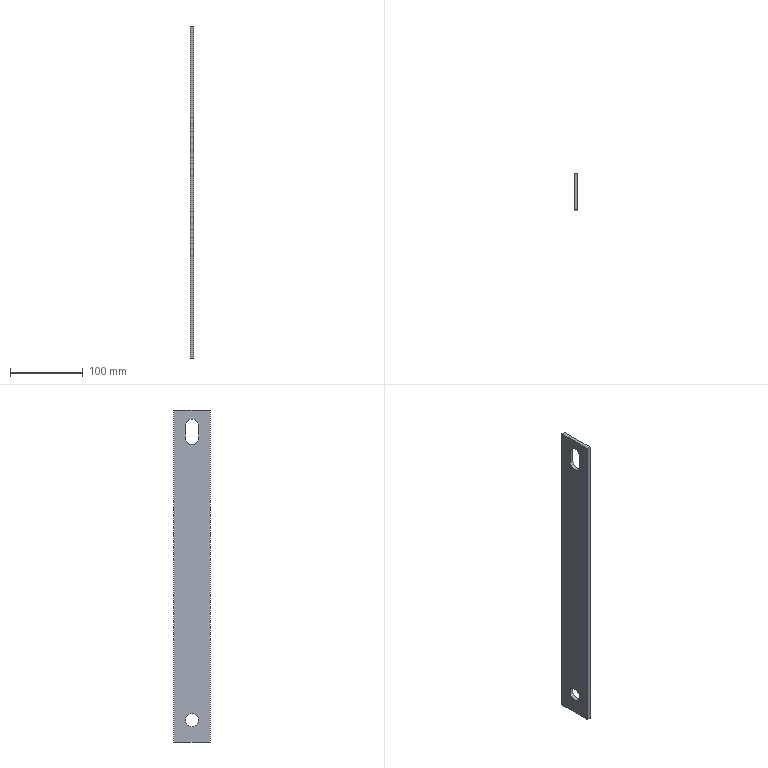Part | NX | features MAIN_BODY 2 | 1 solid | 11 faces | box 5 x 50 x 455 mm | volume 109675 mm3 | plane 8 | cylinder 3 | commonest cylinder face diameters 18 x3
STEP:
#1=CARTESIAN_POINT('',(1560.,-656.,343.5));
#2=VERTEX_POINT('',#1);
#3=CARTESIAN_POINT('',(1560.,-674.,343.5));
#4=VERTEX_POINT('',#3);
#5=CARTESIAN_POINT('',(1560.,-665.,343.5));
#6=DIRECTION('',(-1.,0.,0.));
#7=DIRECTION('',(0.,0.,-1.));
#8=AXIS2_PLACEMENT_3D('',#5,#6,#7);
#9=CIRCLE('',#8,9.);
#10=EDGE_CURVE('',#2,#4,#9,.F.);
#11=ORIENTED_EDGE('',*,*,#10,.F.);
#12=CARTESIAN_POINT('',(1565.,-656.,343.5));
#13=VERTEX_POINT('',#12);
#14=CARTESIAN_POINT('',(1563.,-656.,343.5));
#15=DIRECTION('',(-1.,0.,0.));
#16=VECTOR('',#15,1000.);
#17=LINE('',#14,#16);
#18=EDGE_CURVE('',#13,#2,#17,.T.);
#19=ORIENTED_EDGE('',*,*,#18,.F.);
#20=CARTESIAN_POINT('',(1565.,-674.,343.5));
#21=VERTEX_POINT('',#20);
#22=CARTESIAN_POINT('',(1565.,-665.,343.5));
#23=DIRECTION('',(-1.,0.,0.));
#24=DIRECTION('',(0.,0.,-1.));
#25=AXIS2_PLACEMENT_3D('',#22,#23,#24);
#26=CIRCLE('',#25,9.);
#27=EDGE_CURVE('',#13,#21,#26,.F.);
#28=ORIENTED_EDGE('',*,*,#27,.T.);
#29=CARTESIAN_POINT('',(1563.,-674.,343.5));
#30=DIRECTION('',(-1.,0.,0.));
#31=VECTOR('',#30,1000.);
#32=LINE('',#29,#31);
#33=EDGE_CURVE('',#21,#4,#32,.T.);
#34=ORIENTED_EDGE('',*,*,#33,.T.);
#35=EDGE_LOOP('',(#11,#19,#28,#34));
#36=FACE_BOUND('',#35,.T.);
#37=CARTESIAN_POINT('',(1563.,-665.,343.5));
#38=DIRECTION('',(-1.,0.,0.));
#39=DIRECTION('',(0.,1.,0.));
#40=AXIS2_PLACEMENT_3D('',#37,#38,#39);
#41=CYLINDRICAL_SURFACE('',#40,9.);
#42=ADVANCED_FACE('',(#36),#41,.F.);
#43=CARTESIAN_POINT('',(1560.,-656.,326.5));
#44=VERTEX_POINT('',#43);
#45=CARTESIAN_POINT('',(1560.,-656.,206.25));
#46=DIRECTION('',(0.,0.,-1.));
#47=VECTOR('',#46,1000.);
#48=LINE('',#45,#47);
#49=EDGE_CURVE('',#2,#44,#48,.T.);
#50=ORIENTED_EDGE('',*,*,#49,.T.);
#51=CARTESIAN_POINT('',(1565.,-656.,326.5));
#52=VERTEX_POINT('',#51);
#53=CARTESIAN_POINT('',(1563.,-656.,326.5));
#54=DIRECTION('',(-1.,0.,0.));
#55=VECTOR('',#54,1000.);
#56=LINE('',#53,#55);
#57=EDGE_CURVE('',#52,#44,#56,.T.);
#58=ORIENTED_EDGE('',*,*,#57,.F.);
#59=CARTESIAN_POINT('',(1565.,-656.,206.25));
#60=DIRECTION('',(0.,0.,-1.));
#61=VECTOR('',#60,1000.);
#62=LINE('',#59,#61);
#63=EDGE_CURVE('',#13,#52,#62,.T.);
#64=ORIENTED_EDGE('',*,*,#63,.F.);
#65=ORIENTED_EDGE('',*,*,#18,.T.);
#66=EDGE_LOOP('',(#50,#58,#64,#65));
#67=FACE_BOUND('',#66,.T.);
#68=CARTESIAN_POINT('',(1563.,-656.,206.25));
#69=DIRECTION('',(0.,-1.,0.));
#70=DIRECTION('',(-1.,0.,0.));
#71=AXIS2_PLACEMENT_3D('',#68,#69,#70);
#72=PLANE('',#71);
#73=ADVANCED_FACE('',(#67),#72,.T.);
#74=CARTESIAN_POINT('',(1560.,-674.,326.5));
#75=VERTEX_POINT('',#74);
#76=CARTESIAN_POINT('',(1560.,-665.,326.5));
#77=DIRECTION('',(-1.,0.,0.));
#78=DIRECTION('',(0.,0.,-1.));
#79=AXIS2_PLACEMENT_3D('',#76,#77,#78);
#80=CIRCLE('',#79,9.);
#81=EDGE_CURVE('',#75,#44,#80,.F.);
#82=ORIENTED_EDGE('',*,*,#81,.F.);
#83=CARTESIAN_POINT('',(1565.,-674.,326.5));
#84=VERTEX_POINT('',#83);
#85=CARTESIAN_POINT('',(1563.,-674.,326.5));
#86=DIRECTION('',(1.,0.,0.));
#87=VECTOR('',#86,1000.);
#88=LINE('',#85,#87);
#89=EDGE_CURVE('',#84,#75,#88,.F.);
#90=ORIENTED_EDGE('',*,*,#89,.F.);
#91=CARTESIAN_POINT('',(1565.,-665.,326.5));
#92=DIRECTION('',(-1.,0.,0.));
#93=DIRECTION('',(0.,0.,-1.));
#94=AXIS2_PLACEMENT_3D('',#91,#92,#93);
#95=CIRCLE('',#94,9.);
#96=EDGE_CURVE('',#84,#52,#95,.F.);
#97=ORIENTED_EDGE('',*,*,#96,.T.);
#98=ORIENTED_EDGE('',*,*,#57,.T.);
#99=EDGE_LOOP('',(#82,#90,#97,#98));
#100=FACE_BOUND('',#99,.T.);
#101=CARTESIAN_POINT('',(1563.,-665.,326.5));
#102=DIRECTION('',(-1.,0.,0.));
#103=DIRECTION('',(0.,1.,0.));
#104=AXIS2_PLACEMENT_3D('',#101,#102,#103);
#105=CYLINDRICAL_SURFACE('',#104,9.);
#106=ADVANCED_FACE('',(#100),#105,.F.);
#107=CARTESIAN_POINT('',(1560.,-640.,-90.));
#108=VERTEX_POINT('',#107);
#109=CARTESIAN_POINT('',(1560.,-640.,365.));
#110=VERTEX_POINT('',#109);
#111=CARTESIAN_POINT('',(1560.,-640.,220.));
#112=DIRECTION('',(0.,0.,1.));
#113=VECTOR('',#112,1000.);
#114=LINE('',#111,#113);
#115=EDGE_CURVE('',#108,#110,#114,.T.);
#116=ORIENTED_EDGE('',*,*,#115,.T.);
#117=CARTESIAN_POINT('',(1565.,-640.,365.));
#118=VERTEX_POINT('',#117);
#119=CARTESIAN_POINT('',(1563.,-640.,365.));
#120=DIRECTION('',(-1.,0.,0.));
#121=VECTOR('',#120,1000.);
#122=LINE('',#119,#121);
#123=EDGE_CURVE('',#118,#110,#122,.T.);
#124=ORIENTED_EDGE('',*,*,#123,.F.);
#125=CARTESIAN_POINT('',(1565.,-640.,-90.));
#126=VERTEX_POINT('',#125);
#127=CARTESIAN_POINT('',(1565.,-640.,-80.));
#128=DIRECTION('',(0.,0.,1.));
#129=VECTOR('',#128,1000.);
#130=LINE('',#127,#129);
#131=EDGE_CURVE('',#126,#118,#130,.T.);
#132=ORIENTED_EDGE('',*,*,#131,.F.);
#133=CARTESIAN_POINT('',(1563.,-640.,-90.));
#134=DIRECTION('',(-1.,0.,0.));
#135=VECTOR('',#134,1000.);
#136=LINE('',#133,#135);
#137=EDGE_CURVE('',#126,#108,#136,.T.);
#138=ORIENTED_EDGE('',*,*,#137,.T.);
#139=EDGE_LOOP('',(#116,#124,#132,#138));
#140=FACE_BOUND('',#139,.T.);
#141=CARTESIAN_POINT('',(1563.,-640.,-80.));
#142=DIRECTION('',(0.,1.,0.));
#143=DIRECTION('',(0.,0.,1.));
#144=AXIS2_PLACEMENT_3D('',#141,#142,#143);
#145=PLANE('',#144);
#146=ADVANCED_FACE('',(#140),#145,.T.);
#147=CARTESIAN_POINT('',(1560.,-690.,365.));
#148=VERTEX_POINT('',#147);
#149=CARTESIAN_POINT('',(1560.,-647.5,365.));
#150=DIRECTION('',(0.,-1.,0.));
#151=VECTOR('',#150,1000.);
#152=LINE('',#149,#151);
#153=EDGE_CURVE('',#110,#148,#152,.T.);
#154=ORIENTED_EDGE('',*,*,#153,.T.);
#155=CARTESIAN_POINT('',(1565.,-690.,365.));
#156=VERTEX_POINT('',#155);
#157=CARTESIAN_POINT('',(1563.,-690.,365.));
#158=DIRECTION('',(-1.,0.,0.));
#159=VECTOR('',#158,1000.);
#160=LINE('',#157,#159);
#161=EDGE_CURVE('',#156,#148,#160,.T.);
#162=ORIENTED_EDGE('',*,*,#161,.F.);
#163=CARTESIAN_POINT('',(1565.,-647.5,365.));
#164=DIRECTION('',(0.,-1.,0.));
#165=VECTOR('',#164,1000.);
#166=LINE('',#163,#165);
#167=EDGE_CURVE('',#118,#156,#166,.T.);
#168=ORIENTED_EDGE('',*,*,#167,.F.);
#169=ORIENTED_EDGE('',*,*,#123,.T.);
#170=EDGE_LOOP('',(#154,#162,#168,#169));
#171=FACE_BOUND('',#170,.T.);
#172=CARTESIAN_POINT('',(1563.,-647.5,365.));
#173=DIRECTION('',(0.,0.,1.));
#174=DIRECTION('',(-1.,0.,0.));
#175=AXIS2_PLACEMENT_3D('',#172,#173,#174);
#176=PLANE('',#175);
#177=ADVANCED_FACE('',(#171),#176,.T.);
#178=CARTESIAN_POINT('',(1560.,-690.,-90.));
#179=VERTEX_POINT('',#178);
#180=CARTESIAN_POINT('',(1560.,-690.,220.));
#181=DIRECTION('',(0.,0.,-1.));
#182=VECTOR('',#181,1000.);
#183=LINE('',#180,#182);
#184=EDGE_CURVE('',#148,#179,#183,.T.);
#185=ORIENTED_EDGE('',*,*,#184,.T.);
#186=CARTESIAN_POINT('',(1565.,-690.,-90.));
#187=VERTEX_POINT('',#186);
#188=CARTESIAN_POINT('',(1563.,-690.,-90.));
#189=DIRECTION('',(-1.,0.,0.));
#190=VECTOR('',#189,1000.);
#191=LINE('',#188,#190);
#192=EDGE_CURVE('',#187,#179,#191,.T.);
#193=ORIENTED_EDGE('',*,*,#192,.F.);
#194=CARTESIAN_POINT('',(1565.,-690.,220.));
#195=DIRECTION('',(0.,0.,-1.));
#196=VECTOR('',#195,1000.);
#197=LINE('',#194,#196);
#198=EDGE_CURVE('',#156,#187,#197,.T.);
#199=ORIENTED_EDGE('',*,*,#198,.F.);
#200=ORIENTED_EDGE('',*,*,#161,.T.);
#201=EDGE_LOOP('',(#185,#193,#199,#200));
#202=FACE_BOUND('',#201,.T.);
#203=CARTESIAN_POINT('',(1563.,-690.,220.));
#204=DIRECTION('',(0.,-1.,0.));
#205=DIRECTION('',(0.,0.,-1.));
#206=AXIS2_PLACEMENT_3D('',#203,#204,#205);
#207=PLANE('',#206);
#208=ADVANCED_FACE('',(#202),#207,.T.);
#209=CARTESIAN_POINT('',(1565.,-665.,-69.));
#210=VERTEX_POINT('',#209);
#211=CARTESIAN_POINT('',(1565.,-665.,-60.));
#212=DIRECTION('',(-1.,0.,0.));
#213=DIRECTION('',(0.,0.,-1.));
#214=AXIS2_PLACEMENT_3D('',#211,#212,#213);
#215=CIRCLE('',#214,9.);
#216=EDGE_CURVE('',#210,#210,#215,.F.);
#217=ORIENTED_EDGE('',*,*,#216,.T.);
#218=EDGE_LOOP('',(#217));
#219=FACE_BOUND('',#218,.T.);
#220=CARTESIAN_POINT('',(1560.,-665.,-69.));
#221=VERTEX_POINT('',#220);
#222=CARTESIAN_POINT('',(1560.,-665.,-60.));
#223=DIRECTION('',(-1.,0.,0.));
#224=DIRECTION('',(0.,0.,-1.));
#225=AXIS2_PLACEMENT_3D('',#222,#223,#224);
#226=CIRCLE('',#225,9.);
#227=EDGE_CURVE('',#221,#221,#226,.F.);
#228=ORIENTED_EDGE('',*,*,#227,.F.);
#229=EDGE_LOOP('',(#228));
#230=FACE_BOUND('',#229,.T.);
#231=CARTESIAN_POINT('',(1563.,-665.,-60.));
#232=DIRECTION('',(-1.,0.,0.));
#233=DIRECTION('',(0.,1.,0.));
#234=AXIS2_PLACEMENT_3D('',#231,#232,#233);
#235=CYLINDRICAL_SURFACE('',#234,9.);
#236=ADVANCED_FACE('',(#219,#230),#235,.F.);
#237=CARTESIAN_POINT('',(1560.,-647.5,-90.));
#238=DIRECTION('',(0.,1.,0.));
#239=VECTOR('',#238,1000.);
#240=LINE('',#237,#239);
#241=EDGE_CURVE('',#179,#108,#240,.T.);
#242=ORIENTED_EDGE('',*,*,#241,.T.);
#243=ORIENTED_EDGE('',*,*,#137,.F.);
#244=CARTESIAN_POINT('',(1565.,-682.5,-90.));
#245=DIRECTION('',(0.,1.,0.));
#246=VECTOR('',#245,1000.);
#247=LINE('',#244,#246);
#248=EDGE_CURVE('',#187,#126,#247,.T.);
#249=ORIENTED_EDGE('',*,*,#248,.F.);
#250=ORIENTED_EDGE('',*,*,#192,.T.);
#251=EDGE_LOOP('',(#242,#243,#249,#250));
#252=FACE_BOUND('',#251,.T.);
#253=CARTESIAN_POINT('',(1563.,-682.5,-90.));
#254=DIRECTION('',(0.,0.,-1.));
#255=DIRECTION('',(1.,0.,0.));
#256=AXIS2_PLACEMENT_3D('',#253,#254,#255);
#257=PLANE('',#256);
#258=ADVANCED_FACE('',(#252),#257,.T.);
#259=CARTESIAN_POINT('',(1560.,-674.,193.75));
#260=DIRECTION('',(0.,0.,1.));
#261=VECTOR('',#260,1000.);
#262=LINE('',#259,#261);
#263=EDGE_CURVE('',#75,#4,#262,.T.);
#264=ORIENTED_EDGE('',*,*,#263,.T.);
#265=ORIENTED_EDGE('',*,*,#33,.F.);
#266=CARTESIAN_POINT('',(1565.,-674.,193.75));
#267=DIRECTION('',(0.,0.,1.));
#268=VECTOR('',#267,1000.);
#269=LINE('',#266,#268);
#270=EDGE_CURVE('',#84,#21,#269,.T.);
#271=ORIENTED_EDGE('',*,*,#270,.F.);
#272=ORIENTED_EDGE('',*,*,#89,.T.);
#273=EDGE_LOOP('',(#264,#265,#271,#272));
#274=FACE_BOUND('',#273,.T.);
#275=CARTESIAN_POINT('',(1563.,-674.,193.75));
#276=DIRECTION('',(0.,1.,0.));
#277=DIRECTION('',(1.,0.,0.));
#278=AXIS2_PLACEMENT_3D('',#275,#276,#277);
#279=PLANE('',#278);
#280=ADVANCED_FACE('',(#274),#279,.T.);
#281=ORIENTED_EDGE('',*,*,#131,.T.);
#282=ORIENTED_EDGE('',*,*,#167,.T.);
#283=ORIENTED_EDGE('',*,*,#198,.T.);
#284=ORIENTED_EDGE('',*,*,#248,.T.);
#285=EDGE_LOOP('',(#281,#282,#283,#284));
#286=FACE_BOUND('',#285,.T.);
#287=ORIENTED_EDGE('',*,*,#216,.F.);
#288=EDGE_LOOP('',(#287));
#289=FACE_BOUND('',#288,.T.);
#290=ORIENTED_EDGE('',*,*,#27,.F.);
#291=ORIENTED_EDGE('',*,*,#63,.T.);
#292=ORIENTED_EDGE('',*,*,#96,.F.);
#293=ORIENTED_EDGE('',*,*,#270,.T.);
#294=EDGE_LOOP('',(#290,#291,#292,#293));
#295=FACE_BOUND('',#294,.T.);
#296=CARTESIAN_POINT('',(1565.,-647.5,220.));
#297=DIRECTION('',(-1.,0.,0.));
#298=DIRECTION('',(0.,1.,0.));
#299=AXIS2_PLACEMENT_3D('',#296,#297,#298);
#300=PLANE('',#299);
#301=ADVANCED_FACE('',(#286,#289,#295),#300,.F.);
#302=ORIENTED_EDGE('',*,*,#115,.F.);
#303=ORIENTED_EDGE('',*,*,#241,.F.);
#304=ORIENTED_EDGE('',*,*,#184,.F.);
#305=ORIENTED_EDGE('',*,*,#153,.F.);
#306=EDGE_LOOP('',(#302,#303,#304,#305));
#307=FACE_BOUND('',#306,.T.);
#308=ORIENTED_EDGE('',*,*,#227,.T.);
#309=EDGE_LOOP('',(#308));
#310=FACE_BOUND('',#309,.T.);
#311=ORIENTED_EDGE('',*,*,#10,.T.);
#312=ORIENTED_EDGE('',*,*,#263,.F.);
#313=ORIENTED_EDGE('',*,*,#81,.T.);
#314=ORIENTED_EDGE('',*,*,#49,.F.);
#315=EDGE_LOOP('',(#311,#312,#313,#314));
#316=FACE_BOUND('',#315,.T.);
#317=CARTESIAN_POINT('',(1560.,-647.5,220.));
#318=DIRECTION('',(-1.,0.,0.));
#319=DIRECTION('',(0.,1.,0.));
#320=AXIS2_PLACEMENT_3D('',#317,#318,#319);
#321=PLANE('',#320);
#322=ADVANCED_FACE('',(#307,#310,#316),#321,.T.);
#323=CLOSED_SHELL('',(#42,#73,#106,#146,#177,#208,#236,#258,#280,#301,#322));
#324=MANIFOLD_SOLID_BREP('',#323);
#325=(LENGTH_UNIT()NAMED_UNIT(*)SI_UNIT(.MILLI.,.METRE.));
#326=UNCERTAINTY_MEASURE_WITH_UNIT(LENGTH_MEASURE(0.00001),#325,'','');
#327=(NAMED_UNIT(*)PLANE_ANGLE_UNIT()SI_UNIT($,.RADIAN.));
#328=(NAMED_UNIT(*)SI_UNIT($,.STERADIAN.)SOLID_ANGLE_UNIT());
#329=(GEOMETRIC_REPRESENTATION_CONTEXT(3)GLOBAL_UNCERTAINTY_ASSIGNED_CONTEXT((#326))GLOBAL_UNIT_ASSIGNED_CONTEXT((#325,#327,#328))REPRESENTATION_CONTEXT('',''));
#330=ADVANCED_BREP_SHAPE_REPRESENTATION('',(#324),#329);